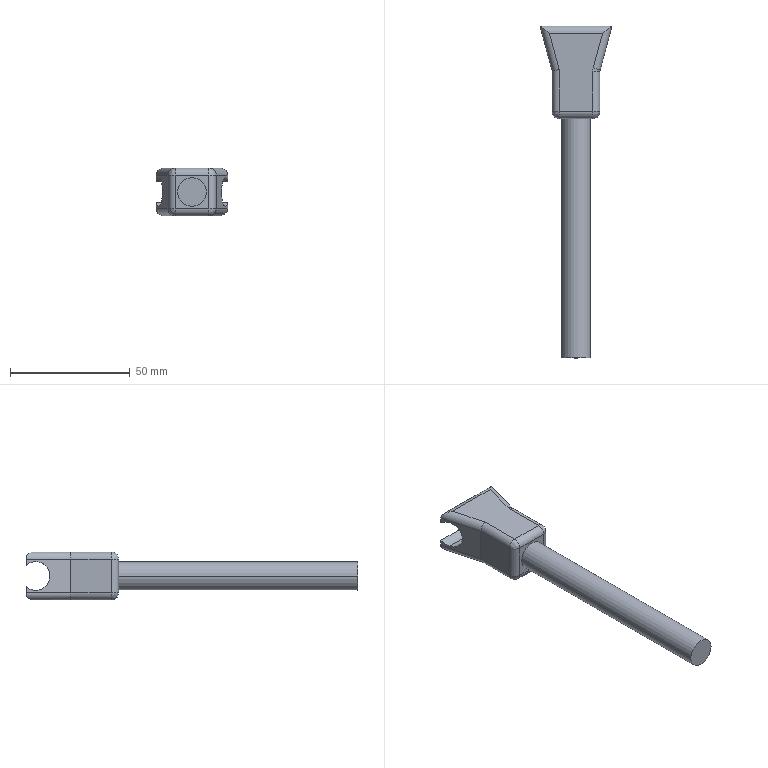Part | SolidWorks | features BaseBody 1 | 1 solid | 36 faces | box 30 x 138.66 x 20 mm | volume 25323 mm3 | cylinder 20 | plane 10 | spline 6 | commonest cylinder face diameters 6 x15 12 x5
STEP:
#1=CARTESIAN_POINT('',(-30.308,-117.701,10.));
#2=VERTEX_POINT('',#1);
#3=CARTESIAN_POINT('',(-18.308,-117.701,10.));
#4=VERTEX_POINT('',#3);
#5=CARTESIAN_POINT('',(-24.308,-117.701,10.));
#6=DIRECTION('',(0.,1.,0.));
#7=DIRECTION('',(-1.,0.,0.));
#8=AXIS2_PLACEMENT_3D('',#5,#6,#7);
#9=CIRCLE('',#8,6.);
#10=EDGE_CURVE('',#2,#4,#9,.T.);
#11=ORIENTED_EDGE('',*,*,#10,.T.);
#12=CARTESIAN_POINT('',(-18.308,-17.701,10.));
#13=VERTEX_POINT('',#12);
#14=CARTESIAN_POINT('',(-18.308,-117.701,10.));
#15=DIRECTION('',(0.,1.,0.));
#16=VECTOR('',#15,1000.);
#17=LINE('',#14,#16);
#18=EDGE_CURVE('',#4,#13,#17,.T.);
#19=ORIENTED_EDGE('',*,*,#18,.T.);
#20=CARTESIAN_POINT('',(-30.308,-17.701,10.));
#21=VERTEX_POINT('',#20);
#22=CARTESIAN_POINT('',(-24.308,-17.701,10.));
#23=DIRECTION('',(0.,-1.,0.));
#24=DIRECTION('',(-1.,0.,0.));
#25=AXIS2_PLACEMENT_3D('',#22,#23,#24);
#26=CIRCLE('',#25,6.);
#27=EDGE_CURVE('',#13,#21,#26,.T.);
#28=ORIENTED_EDGE('',*,*,#27,.T.);
#29=CARTESIAN_POINT('',(-30.308,-117.701,10.));
#30=DIRECTION('',(0.,1.,0.));
#31=VECTOR('',#30,1000.);
#32=LINE('',#29,#31);
#33=EDGE_CURVE('',#2,#21,#32,.T.);
#34=ORIENTED_EDGE('',*,*,#33,.F.);
#35=EDGE_LOOP('',(#11,#19,#28,#34));
#36=FACE_OUTER_BOUND('',#35,.T.);
#37=CARTESIAN_POINT('',(-24.308,-117.701,10.));
#38=DIRECTION('',(0.,1.,0.));
#39=DIRECTION('',(-1.,0.,0.));
#40=AXIS2_PLACEMENT_3D('',#37,#38,#39);
#41=CYLINDRICAL_SURFACE('',#40,6.);
#42=ADVANCED_FACE('',(#36),#41,.T.);
#43=CARTESIAN_POINT('',(-38.236,16.959,4.));
#44=VERTEX_POINT('',#43);
#45=CARTESIAN_POINT('',(-38.236,16.959,16.));
#46=VERTEX_POINT('',#45);
#47=CARTESIAN_POINT('',(-38.236,16.959,4.));
#48=CARTESIAN_POINT('',(-35.021,4.959,4.));
#49=CARTESIAN_POINT('',(-35.021,4.959,16.));
#50=CARTESIAN_POINT('',(-38.236,16.959,16.));
#51=(BOUNDED_CURVE()B_SPLINE_CURVE(3,(#47,#48,#49,#50),.UNSPECIFIED.,.F.,.F.)B_SPLINE_CURVE_WITH_KNOTS((4,4),(4.712,7.854),.UNSPECIFIED.)CURVE()GEOMETRIC_REPRESENTATION_ITEM()RATIONAL_B_SPLINE_CURVE((1.,0.3333,0.3333,1.))REPRESENTATION_ITEM(''));
#52=EDGE_CURVE('',#44,#46,#51,.T.);
#53=ORIENTED_EDGE('',*,*,#52,.T.);
#54=CARTESIAN_POINT('',(-10.38,16.959,16.));
#55=VERTEX_POINT('',#54);
#56=CARTESIAN_POINT('',(-100.,16.959,16.));
#57=DIRECTION('',(1.,0.,0.));
#58=VECTOR('',#57,1000.);
#59=LINE('',#56,#58);
#60=EDGE_CURVE('',#46,#55,#59,.T.);
#61=ORIENTED_EDGE('',*,*,#60,.T.);
#62=CARTESIAN_POINT('',(-10.38,16.959,4.));
#63=VERTEX_POINT('',#62);
#64=CARTESIAN_POINT('',(-10.38,16.959,16.));
#65=CARTESIAN_POINT('',(-13.595,4.959,16.));
#66=CARTESIAN_POINT('',(-13.595,4.959,4.));
#67=CARTESIAN_POINT('',(-10.38,16.959,4.));
#68=(BOUNDED_CURVE()B_SPLINE_CURVE(3,(#64,#65,#66,#67),.UNSPECIFIED.,.F.,.F.)B_SPLINE_CURVE_WITH_KNOTS((4,4),(1.571,4.712),.UNSPECIFIED.)CURVE()GEOMETRIC_REPRESENTATION_ITEM()RATIONAL_B_SPLINE_CURVE((1.,0.3333,0.3333,1.))REPRESENTATION_ITEM(''));
#69=EDGE_CURVE('',#55,#63,#68,.T.);
#70=ORIENTED_EDGE('',*,*,#69,.T.);
#71=CARTESIAN_POINT('',(-100.,16.959,4.));
#72=DIRECTION('',(1.,0.,0.));
#73=VECTOR('',#72,1000.);
#74=LINE('',#71,#73);
#75=EDGE_CURVE('',#44,#63,#74,.T.);
#76=ORIENTED_EDGE('',*,*,#75,.F.);
#77=EDGE_LOOP('',(#53,#61,#70,#76));
#78=FACE_OUTER_BOUND('',#77,.T.);
#79=CARTESIAN_POINT('',(-100.,16.959,10.));
#80=DIRECTION('',(1.,0.,0.));
#81=DIRECTION('',(0.,0.,-1.));
#82=AXIS2_PLACEMENT_3D('',#79,#80,#81);
#83=CYLINDRICAL_SURFACE('',#82,6.);
#84=ADVANCED_FACE('',(#78),#83,.F.);
#85=CARTESIAN_POINT('',(-39.308,20.959,5.528));
#86=VERTEX_POINT('',#85);
#87=CARTESIAN_POINT('',(-39.308,20.959,5.528));
#88=CARTESIAN_POINT('',(-39.01,19.847,4.533));
#89=CARTESIAN_POINT('',(-38.636,18.452,4.));
#90=CARTESIAN_POINT('',(-38.236,16.959,4.));
#91=(BOUNDED_CURVE()B_SPLINE_CURVE(3,(#87,#88,#89,#90),.UNSPECIFIED.,.F.,.T.)B_SPLINE_CURVE_WITH_KNOTS((4,4),(3.983,4.712),.UNSPECIFIED.)CURVE()GEOMETRIC_REPRESENTATION_ITEM()RATIONAL_B_SPLINE_CURVE((1.,0.9561,0.9561,1.))REPRESENTATION_ITEM(''));
#92=EDGE_CURVE('',#86,#44,#91,.T.);
#93=ORIENTED_EDGE('',*,*,#92,.T.);
#94=ORIENTED_EDGE('',*,*,#75,.T.);
#95=CARTESIAN_POINT('',(-9.308,20.959,5.528));
#96=VERTEX_POINT('',#95);
#97=CARTESIAN_POINT('',(-10.38,16.959,4.));
#98=CARTESIAN_POINT('',(-9.98,18.452,4.));
#99=CARTESIAN_POINT('',(-9.606,19.847,4.533));
#100=CARTESIAN_POINT('',(-9.308,20.959,5.528));
#101=(BOUNDED_CURVE()B_SPLINE_CURVE(3,(#97,#98,#99,#100),.UNSPECIFIED.,.F.,.F.)B_SPLINE_CURVE_WITH_KNOTS((4,4),(4.712,5.442),.UNSPECIFIED.)CURVE()GEOMETRIC_REPRESENTATION_ITEM()RATIONAL_B_SPLINE_CURVE((1.,0.9561,0.9561,1.))REPRESENTATION_ITEM(''));
#102=EDGE_CURVE('',#63,#96,#101,.T.);
#103=ORIENTED_EDGE('',*,*,#102,.T.);
#104=CARTESIAN_POINT('',(-39.308,20.959,5.528));
#105=DIRECTION('',(-1.,0.,0.));
#106=VECTOR('',#105,1000.);
#107=LINE('',#104,#106);
#108=EDGE_CURVE('',#96,#86,#107,.T.);
#109=ORIENTED_EDGE('',*,*,#108,.T.);
#110=EDGE_LOOP('',(#93,#94,#103,#109));
#111=FACE_OUTER_BOUND('',#110,.T.);
#112=CARTESIAN_POINT('',(-100.,16.959,10.));
#113=DIRECTION('',(1.,0.,0.));
#114=DIRECTION('',(0.,0.,-1.));
#115=AXIS2_PLACEMENT_3D('',#112,#113,#114);
#116=CYLINDRICAL_SURFACE('',#115,6.);
#117=ADVANCED_FACE('',(#111),#116,.F.);
#118=ORIENTED_EDGE('',*,*,#18,.F.);
#119=CARTESIAN_POINT('',(-24.308,-117.701,10.));
#120=DIRECTION('',(0.,1.,0.));
#121=DIRECTION('',(-1.,0.,0.));
#122=AXIS2_PLACEMENT_3D('',#119,#120,#121);
#123=CIRCLE('',#122,6.);
#124=EDGE_CURVE('',#4,#2,#123,.T.);
#125=ORIENTED_EDGE('',*,*,#124,.T.);
#126=ORIENTED_EDGE('',*,*,#33,.T.);
#127=CARTESIAN_POINT('',(-24.308,-17.701,10.));
#128=DIRECTION('',(0.,-1.,0.));
#129=DIRECTION('',(-1.,0.,0.));
#130=AXIS2_PLACEMENT_3D('',#127,#128,#129);
#131=CIRCLE('',#130,6.);
#132=EDGE_CURVE('',#21,#13,#131,.T.);
#133=ORIENTED_EDGE('',*,*,#132,.T.);
#134=EDGE_LOOP('',(#118,#125,#126,#133));
#135=FACE_OUTER_BOUND('',#134,.T.);
#136=CARTESIAN_POINT('',(-24.308,-117.701,10.));
#137=DIRECTION('',(0.,1.,0.));
#138=DIRECTION('',(-1.,0.,0.));
#139=AXIS2_PLACEMENT_3D('',#136,#137,#138);
#140=CYLINDRICAL_SURFACE('',#139,6.);
#141=ADVANCED_FACE('',(#135),#140,.T.);
#142=ORIENTED_EDGE('',*,*,#132,.F.);
#143=ORIENTED_EDGE('',*,*,#27,.F.);
#144=EDGE_LOOP('',(#142,#143));
#145=FACE_BOUND('',#144,.T.);
#146=CARTESIAN_POINT('',(-31.308,-17.701,3.));
#147=VERTEX_POINT('',#146);
#148=CARTESIAN_POINT('',(-31.308,-17.701,17.));
#149=VERTEX_POINT('',#148);
#150=CARTESIAN_POINT('',(-31.308,-17.701,20.));
#151=DIRECTION('',(0.,0.,1.));
#152=VECTOR('',#151,1000.);
#153=LINE('',#150,#152);
#154=EDGE_CURVE('',#147,#149,#153,.T.);
#155=ORIENTED_EDGE('',*,*,#154,.F.);
#156=CARTESIAN_POINT('',(-17.308,-17.701,3.));
#157=VERTEX_POINT('',#156);
#158=CARTESIAN_POINT('',(-14.308,-17.701,3.));
#159=DIRECTION('',(-1.,0.,0.));
#160=VECTOR('',#159,1000.);
#161=LINE('',#158,#160);
#162=EDGE_CURVE('',#157,#147,#161,.T.);
#163=ORIENTED_EDGE('',*,*,#162,.F.);
#164=CARTESIAN_POINT('',(-17.308,-17.701,17.));
#165=VERTEX_POINT('',#164);
#166=CARTESIAN_POINT('',(-17.308,-17.701,20.));
#167=DIRECTION('',(0.,0.,-1.));
#168=VECTOR('',#167,1000.);
#169=LINE('',#166,#168);
#170=EDGE_CURVE('',#165,#157,#169,.T.);
#171=ORIENTED_EDGE('',*,*,#170,.F.);
#172=CARTESIAN_POINT('',(-14.308,-17.701,17.));
#173=DIRECTION('',(1.,0.,0.));
#174=VECTOR('',#173,1000.);
#175=LINE('',#172,#174);
#176=EDGE_CURVE('',#149,#165,#175,.T.);
#177=ORIENTED_EDGE('',*,*,#176,.F.);
#178=EDGE_LOOP('',(#155,#163,#171,#177));
#179=FACE_OUTER_BOUND('',#178,.T.);
#180=CARTESIAN_POINT('',(-14.308,-17.701,20.));
#181=DIRECTION('',(0.,1.,0.));
#182=DIRECTION('',(-1.,0.,0.));
#183=AXIS2_PLACEMENT_3D('',#180,#181,#182);
#184=PLANE('',#183);
#185=ADVANCED_FACE('',(#145,#179),#184,.F.);
#186=ORIENTED_EDGE('',*,*,#10,.F.);
#187=ORIENTED_EDGE('',*,*,#124,.F.);
#188=EDGE_LOOP('',(#186,#187));
#189=FACE_OUTER_BOUND('',#188,.T.);
#190=CARTESIAN_POINT('',(-24.308,-117.701,10.));
#191=DIRECTION('',(0.,-1.,0.));
#192=DIRECTION('',(1.,0.,0.));
#193=AXIS2_PLACEMENT_3D('',#190,#191,#192);
#194=PLANE('',#193);
#195=ADVANCED_FACE('',(#189),#194,.T.);
#196=CARTESIAN_POINT('',(-17.308,-14.701,20.));
#197=VERTEX_POINT('',#196);
#198=CARTESIAN_POINT('',(-17.308,-14.701,17.));
#199=DIRECTION('',(-1.,0.,0.));
#200=DIRECTION('',(0.,1.,0.));
#201=AXIS2_PLACEMENT_3D('',#198,#199,#200);
#202=CIRCLE('',#201,3.);
#203=EDGE_CURVE('',#165,#197,#202,.T.);
#204=ORIENTED_EDGE('',*,*,#203,.T.);
#205=CARTESIAN_POINT('',(-31.308,-14.701,20.));
#206=VERTEX_POINT('',#205);
#207=CARTESIAN_POINT('',(0.,-14.701,20.));
#208=DIRECTION('',(-1.,0.,0.));
#209=VECTOR('',#208,1000.);
#210=LINE('',#207,#209);
#211=EDGE_CURVE('',#197,#206,#210,.T.);
#212=ORIENTED_EDGE('',*,*,#211,.T.);
#213=CARTESIAN_POINT('',(-31.308,-14.701,17.));
#214=DIRECTION('',(1.,0.,0.));
#215=DIRECTION('',(0.,1.,0.));
#216=AXIS2_PLACEMENT_3D('',#213,#214,#215);
#217=CIRCLE('',#216,3.);
#218=EDGE_CURVE('',#206,#149,#217,.T.);
#219=ORIENTED_EDGE('',*,*,#218,.T.);
#220=ORIENTED_EDGE('',*,*,#176,.T.);
#221=EDGE_LOOP('',(#204,#212,#219,#220));
#222=FACE_OUTER_BOUND('',#221,.T.);
#223=CARTESIAN_POINT('',(0.,-14.701,17.));
#224=DIRECTION('',(1.,0.,0.));
#225=DIRECTION('',(0.,1.,0.));
#226=AXIS2_PLACEMENT_3D('',#223,#224,#225);
#227=CYLINDRICAL_SURFACE('',#226,3.);
#228=ADVANCED_FACE('',(#222),#227,.T.);
#229=CARTESIAN_POINT('',(-34.308,-14.701,17.));
#230=VERTEX_POINT('',#229);
#231=CARTESIAN_POINT('',(-31.308,-14.701,17.));
#232=DIRECTION('',(0.,0.,-1.));
#233=DIRECTION('',(-1.,0.,0.));
#234=AXIS2_PLACEMENT_3D('',#231,#232,#233);
#235=CIRCLE('',#234,3.);
#236=EDGE_CURVE('',#149,#230,#235,.T.);
#237=ORIENTED_EDGE('',*,*,#236,.T.);
#238=CARTESIAN_POINT('',(-34.308,-14.701,3.));
#239=VERTEX_POINT('',#238);
#240=CARTESIAN_POINT('',(-34.308,-14.701,20.));
#241=DIRECTION('',(0.,0.,-1.));
#242=VECTOR('',#241,1000.);
#243=LINE('',#240,#242);
#244=EDGE_CURVE('',#230,#239,#243,.T.);
#245=ORIENTED_EDGE('',*,*,#244,.T.);
#246=CARTESIAN_POINT('',(-31.308,-14.701,3.));
#247=DIRECTION('',(0.,0.,1.));
#248=DIRECTION('',(-1.,0.,0.));
#249=AXIS2_PLACEMENT_3D('',#246,#247,#248);
#250=CIRCLE('',#249,3.);
#251=EDGE_CURVE('',#239,#147,#250,.T.);
#252=ORIENTED_EDGE('',*,*,#251,.T.);
#253=ORIENTED_EDGE('',*,*,#154,.T.);
#254=EDGE_LOOP('',(#237,#245,#252,#253));
#255=FACE_OUTER_BOUND('',#254,.T.);
#256=CARTESIAN_POINT('',(-31.308,-14.701,20.));
#257=DIRECTION('',(0.,0.,-1.));
#258=DIRECTION('',(-1.,0.,0.));
#259=AXIS2_PLACEMENT_3D('',#256,#257,#258);
#260=CYLINDRICAL_SURFACE('',#259,3.);
#261=ADVANCED_FACE('',(#255),#260,.T.);
#262=CARTESIAN_POINT('',(-17.308,-14.701,0.));
#263=VERTEX_POINT('',#262);
#264=CARTESIAN_POINT('',(-17.308,-14.701,3.));
#265=DIRECTION('',(-1.,0.,0.));
#266=DIRECTION('',(0.,-1.,0.));
#267=AXIS2_PLACEMENT_3D('',#264,#265,#266);
#268=CIRCLE('',#267,3.);
#269=EDGE_CURVE('',#263,#157,#268,.T.);
#270=ORIENTED_EDGE('',*,*,#269,.T.);
#271=ORIENTED_EDGE('',*,*,#162,.T.);
#272=CARTESIAN_POINT('',(-31.308,-14.701,0.));
#273=VERTEX_POINT('',#272);
#274=CARTESIAN_POINT('',(-31.308,-14.701,3.));
#275=DIRECTION('',(1.,0.,0.));
#276=DIRECTION('',(0.,-1.,0.));
#277=AXIS2_PLACEMENT_3D('',#274,#275,#276);
#278=CIRCLE('',#277,3.);
#279=EDGE_CURVE('',#147,#273,#278,.T.);
#280=ORIENTED_EDGE('',*,*,#279,.T.);
#281=CARTESIAN_POINT('',(-14.308,-14.701,0.));
#282=DIRECTION('',(1.,0.,0.));
#283=VECTOR('',#282,1000.);
#284=LINE('',#281,#283);
#285=EDGE_CURVE('',#273,#263,#284,.T.);
#286=ORIENTED_EDGE('',*,*,#285,.T.);
#287=EDGE_LOOP('',(#270,#271,#280,#286));
#288=FACE_OUTER_BOUND('',#287,.T.);
#289=CARTESIAN_POINT('',(-14.308,-14.701,3.));
#290=DIRECTION('',(-1.,0.,0.));
#291=DIRECTION('',(0.,-1.,0.));
#292=AXIS2_PLACEMENT_3D('',#289,#290,#291);
#293=CYLINDRICAL_SURFACE('',#292,3.);
#294=ADVANCED_FACE('',(#288),#293,.T.);
#295=CARTESIAN_POINT('',(-14.308,-14.701,17.));
#296=VERTEX_POINT('',#295);
#297=CARTESIAN_POINT('',(-17.308,-14.701,17.));
#298=DIRECTION('',(0.,0.,-1.));
#299=DIRECTION('',(-1.,0.,0.));
#300=AXIS2_PLACEMENT_3D('',#297,#298,#299);
#301=CIRCLE('',#300,3.);
#302=EDGE_CURVE('',#296,#165,#301,.T.);
#303=ORIENTED_EDGE('',*,*,#302,.T.);
#304=ORIENTED_EDGE('',*,*,#170,.T.);
#305=CARTESIAN_POINT('',(-14.308,-14.701,3.));
#306=VERTEX_POINT('',#305);
#307=CARTESIAN_POINT('',(-17.308,-14.701,3.));
#308=DIRECTION('',(0.,0.,1.));
#309=DIRECTION('',(-1.,0.,0.));
#310=AXIS2_PLACEMENT_3D('',#307,#308,#309);
#311=CIRCLE('',#310,3.);
#312=EDGE_CURVE('',#157,#306,#311,.T.);
#313=ORIENTED_EDGE('',*,*,#312,.T.);
#314=CARTESIAN_POINT('',(-14.308,-14.701,20.));
#315=DIRECTION('',(0.,0.,1.));
#316=VECTOR('',#315,1000.);
#317=LINE('',#314,#316);
#318=EDGE_CURVE('',#306,#296,#317,.T.);
#319=ORIENTED_EDGE('',*,*,#318,.T.);
#320=EDGE_LOOP('',(#303,#304,#313,#319));
#321=FACE_OUTER_BOUND('',#320,.T.);
#322=CARTESIAN_POINT('',(-17.308,-14.701,20.));
#323=DIRECTION('',(0.,0.,-1.));
#324=DIRECTION('',(-1.,0.,0.));
#325=AXIS2_PLACEMENT_3D('',#322,#323,#324);
#326=CYLINDRICAL_SURFACE('',#325,3.);
#327=ADVANCED_FACE('',(#321),#326,.T.);
#328=CARTESIAN_POINT('',(-13.218,17.959,20.));
#329=VERTEX_POINT('',#328);
#330=CARTESIAN_POINT('',(-17.104,3.457,20.));
#331=VERTEX_POINT('',#330);
#332=CARTESIAN_POINT('',(-13.218,17.959,20.));
#333=DIRECTION('',(-0.2588,-0.9659,0.));
#334=VECTOR('',#333,1000.);
#335=LINE('',#332,#334);
#336=EDGE_CURVE('',#329,#331,#335,.T.);
#337=ORIENTED_EDGE('',*,*,#336,.F.);
#338=CARTESIAN_POINT('',(-35.399,17.959,20.));
#339=VERTEX_POINT('',#338);
#340=CARTESIAN_POINT('',(0.,17.959,20.));
#341=DIRECTION('',(1.,0.,0.));
#342=VECTOR('',#341,1000.);
#343=LINE('',#340,#342);
#344=EDGE_CURVE('',#339,#329,#343,.T.);
#345=ORIENTED_EDGE('',*,*,#344,.F.);
#346=CARTESIAN_POINT('',(-31.308,2.694,20.));
#347=VERTEX_POINT('',#346);
#348=CARTESIAN_POINT('',(-31.308,2.694,20.));
#349=DIRECTION('',(-0.2588,0.9659,0.));
#350=VECTOR('',#349,1000.);
#351=LINE('',#348,#350);
#352=EDGE_CURVE('',#347,#339,#351,.T.);
#353=ORIENTED_EDGE('',*,*,#352,.F.);
#354=CARTESIAN_POINT('',(-31.308,0.,20.));
#355=DIRECTION('',(0.,1.,0.));
#356=VECTOR('',#355,1000.);
#357=LINE('',#354,#356);
#358=EDGE_CURVE('',#206,#347,#357,.T.);
#359=ORIENTED_EDGE('',*,*,#358,.F.);
#360=ORIENTED_EDGE('',*,*,#211,.F.);
#361=CARTESIAN_POINT('',(-17.308,1.904,20.));
#362=VERTEX_POINT('',#361);
#363=CARTESIAN_POINT('',(-17.308,0.,20.));
#364=DIRECTION('',(0.,-1.,0.));
#365=VECTOR('',#364,1000.);
#366=LINE('',#363,#365);
#367=EDGE_CURVE('',#362,#197,#366,.T.);
#368=ORIENTED_EDGE('',*,*,#367,.F.);
#369=CARTESIAN_POINT('',(-17.104,3.457,20.));
#370=CARTESIAN_POINT('',(-17.24,2.95,20.));
#371=CARTESIAN_POINT('',(-17.308,2.429,20.));
#372=CARTESIAN_POINT('',(-17.308,1.904,20.));
#373=(BOUNDED_CURVE()B_SPLINE_CURVE(3,(#369,#370,#371,#372),.UNSPECIFIED.,.F.,.F.)B_SPLINE_CURVE_WITH_KNOTS((4,4),(0.,1.),.UNSPECIFIED.)CURVE()GEOMETRIC_REPRESENTATION_ITEM()RATIONAL_B_SPLINE_CURVE((1.,0.9943,0.9943,1.))REPRESENTATION_ITEM(''));
#374=EDGE_CURVE('',#331,#362,#373,.T.);
#375=ORIENTED_EDGE('',*,*,#374,.F.);
#376=EDGE_LOOP('',(#337,#345,#353,#359,#360,#368,#375));
#377=FACE_OUTER_BOUND('',#376,.T.);
#378=CARTESIAN_POINT('',(0.,0.,20.));
#379=DIRECTION('',(0.,0.,-1.));
#380=DIRECTION('',(-1.,0.,0.));
#381=AXIS2_PLACEMENT_3D('',#378,#379,#380);
#382=PLANE('',#381);
#383=ADVANCED_FACE('',(#377),#382,.F.);
#384=ORIENTED_EDGE('',*,*,#302,.F.);
#385=CARTESIAN_POINT('',(-17.308,-14.701,17.));
#386=DIRECTION('',(0.,-1.,0.));
#387=DIRECTION('',(1.,0.,0.));
#388=AXIS2_PLACEMENT_3D('',#385,#386,#387);
#389=CIRCLE('',#388,3.);
#390=EDGE_CURVE('',#296,#197,#389,.T.);
#391=ORIENTED_EDGE('',*,*,#390,.T.);
#392=ORIENTED_EDGE('',*,*,#203,.F.);
#393=EDGE_LOOP('',(#384,#391,#392));
#394=FACE_OUTER_BOUND('',#393,.T.);
#395=CARTESIAN_POINT('',(-14.308,-14.701,17.));
#396=CARTESIAN_POINT('',(-14.308,-14.701,17.));
#397=CARTESIAN_POINT('',(-14.308,-14.701,17.));
#398=CARTESIAN_POINT('',(-14.308,-14.701,17.));
#399=CARTESIAN_POINT('',(-14.308,-14.701,18.757));
#400=CARTESIAN_POINT('',(-14.308,-15.73,18.757));
#401=CARTESIAN_POINT('',(-14.308,-16.458,18.029));
#402=CARTESIAN_POINT('',(-14.308,-16.458,17.));
#403=CARTESIAN_POINT('',(-15.551,-14.701,20.));
#404=CARTESIAN_POINT('',(-15.551,-16.458,20.));
#405=CARTESIAN_POINT('',(-15.551,-17.701,18.757));
#406=CARTESIAN_POINT('',(-15.551,-17.701,17.));
#407=CARTESIAN_POINT('',(-17.308,-14.701,20.));
#408=CARTESIAN_POINT('',(-17.308,-16.458,20.));
#409=CARTESIAN_POINT('',(-17.308,-17.701,18.757));
#410=CARTESIAN_POINT('',(-17.308,-17.701,17.));
#411=(BOUNDED_SURFACE()B_SPLINE_SURFACE(3,3,((#395,#396,#397,#398),(#399,#400,#401,#402),(#403,#404,#405,#406),(#407,#408,#409,#410)),.UNSPECIFIED.,.F.,.F.,.T.)B_SPLINE_SURFACE_WITH_KNOTS((4,4),(4,4),(0.,1.),(0.,1.),.UNSPECIFIED.)GEOMETRIC_REPRESENTATION_ITEM()RATIONAL_B_SPLINE_SURFACE(((1.,0.8047,0.8047,1.),(0.8047,0.6476,0.6476,0.8047),(0.8047,0.6476,0.6476,0.8047),(1.,0.8047,0.8047,1.)))REPRESENTATION_ITEM('')SURFACE());
#412=ADVANCED_FACE('',(#394),#411,.T.);
#413=ORIENTED_EDGE('',*,*,#218,.F.);
#414=CARTESIAN_POINT('',(-31.308,-14.701,17.));
#415=DIRECTION('',(0.,-1.,0.));
#416=DIRECTION('',(1.,0.,0.));
#417=AXIS2_PLACEMENT_3D('',#414,#415,#416);
#418=CIRCLE('',#417,3.);
#419=EDGE_CURVE('',#206,#230,#418,.T.);
#420=ORIENTED_EDGE('',*,*,#419,.T.);
#421=ORIENTED_EDGE('',*,*,#236,.F.);
#422=EDGE_LOOP('',(#413,#420,#421));
#423=FACE_OUTER_BOUND('',#422,.T.);
#424=CARTESIAN_POINT('',(-31.308,-14.701,20.));
#425=CARTESIAN_POINT('',(-31.308,-16.458,20.));
#426=CARTESIAN_POINT('',(-31.308,-17.701,18.757));
#427=CARTESIAN_POINT('',(-31.308,-17.701,17.));
#428=CARTESIAN_POINT('',(-33.066,-14.701,20.));
#429=CARTESIAN_POINT('',(-33.066,-16.458,20.));
#430=CARTESIAN_POINT('',(-33.066,-17.701,18.757));
#431=CARTESIAN_POINT('',(-33.066,-17.701,17.));
#432=CARTESIAN_POINT('',(-34.308,-14.701,18.757));
#433=CARTESIAN_POINT('',(-34.308,-15.73,18.757));
#434=CARTESIAN_POINT('',(-34.308,-16.458,18.029));
#435=CARTESIAN_POINT('',(-34.308,-16.458,17.));
#436=CARTESIAN_POINT('',(-34.308,-14.701,17.));
#437=CARTESIAN_POINT('',(-34.308,-14.701,17.));
#438=CARTESIAN_POINT('',(-34.308,-14.701,17.));
#439=CARTESIAN_POINT('',(-34.308,-14.701,17.));
#440=(BOUNDED_SURFACE()B_SPLINE_SURFACE(3,3,((#424,#425,#426,#427),(#428,#429,#430,#431),(#432,#433,#434,#435),(#436,#437,#438,#439)),.UNSPECIFIED.,.F.,.F.,.F.)B_SPLINE_SURFACE_WITH_KNOTS((4,4),(4,4),(0.,1.),(0.,1.),.UNSPECIFIED.)GEOMETRIC_REPRESENTATION_ITEM()RATIONAL_B_SPLINE_SURFACE(((1.,0.8047,0.8047,1.),(0.8047,0.6476,0.6476,0.8047),(0.8047,0.6476,0.6476,0.8047),(1.,0.8047,0.8047,1.)))REPRESENTATION_ITEM('')SURFACE());
#441=ADVANCED_FACE('',(#423),#440,.T.);
#442=CARTESIAN_POINT('',(-34.308,2.299,17.));
#443=VERTEX_POINT('',#442);
#444=CARTESIAN_POINT('',(-34.308,-17.701,17.));
#445=DIRECTION('',(0.,-1.,0.));
#446=VECTOR('',#445,1000.);
#447=LINE('',#444,#446);
#448=EDGE_CURVE('',#443,#230,#447,.T.);
#449=ORIENTED_EDGE('',*,*,#448,.F.);
#450=CARTESIAN_POINT('',(-34.308,2.299,3.));
#451=VERTEX_POINT('',#450);
#452=CARTESIAN_POINT('',(-34.308,2.299,20.));
#453=DIRECTION('',(0.,0.,1.));
#454=VECTOR('',#453,1000.);
#455=LINE('',#452,#454);
#456=EDGE_CURVE('',#451,#443,#455,.T.);
#457=ORIENTED_EDGE('',*,*,#456,.F.);
#458=CARTESIAN_POINT('',(-34.308,-17.701,3.));
#459=DIRECTION('',(0.,1.,0.));
#460=VECTOR('',#459,1000.);
#461=LINE('',#458,#460);
#462=EDGE_CURVE('',#239,#451,#461,.T.);
#463=ORIENTED_EDGE('',*,*,#462,.F.);
#464=ORIENTED_EDGE('',*,*,#244,.F.);
#465=EDGE_LOOP('',(#449,#457,#463,#464));
#466=FACE_OUTER_BOUND('',#465,.T.);
#467=CARTESIAN_POINT('',(-34.308,-17.701,20.));
#468=DIRECTION('',(1.,0.,0.));
#469=DIRECTION('',(0.,0.,-1.));
#470=AXIS2_PLACEMENT_3D('',#467,#468,#469);
#471=PLANE('',#470);
#472=ADVANCED_FACE('',(#466),#471,.F.);
#473=ORIENTED_EDGE('',*,*,#279,.F.);
#474=ORIENTED_EDGE('',*,*,#251,.F.);
#475=CARTESIAN_POINT('',(-31.308,-14.701,3.));
#476=DIRECTION('',(0.,-1.,0.));
#477=DIRECTION('',(1.,0.,0.));
#478=AXIS2_PLACEMENT_3D('',#475,#476,#477);
#479=CIRCLE('',#478,3.);
#480=EDGE_CURVE('',#239,#273,#479,.T.);
#481=ORIENTED_EDGE('',*,*,#480,.T.);
#482=EDGE_LOOP('',(#473,#474,#481));
#483=FACE_OUTER_BOUND('',#482,.T.);
#484=CARTESIAN_POINT('',(-31.308,-17.701,3.));
#485=CARTESIAN_POINT('',(-31.308,-17.701,1.243));
#486=CARTESIAN_POINT('',(-31.308,-16.458,0.));
#487=CARTESIAN_POINT('',(-31.308,-14.701,0.));
#488=CARTESIAN_POINT('',(-33.066,-17.701,3.));
#489=CARTESIAN_POINT('',(-33.066,-17.701,1.243));
#490=CARTESIAN_POINT('',(-33.066,-16.458,0.));
#491=CARTESIAN_POINT('',(-33.066,-14.701,0.));
#492=CARTESIAN_POINT('',(-34.308,-16.458,3.));
#493=CARTESIAN_POINT('',(-34.308,-16.458,1.971));
#494=CARTESIAN_POINT('',(-34.308,-15.73,1.243));
#495=CARTESIAN_POINT('',(-34.308,-14.701,1.243));
#496=CARTESIAN_POINT('',(-34.308,-14.701,3.));
#497=CARTESIAN_POINT('',(-34.308,-14.701,3.));
#498=CARTESIAN_POINT('',(-34.308,-14.701,3.));
#499=CARTESIAN_POINT('',(-34.308,-14.701,3.));
#500=(BOUNDED_SURFACE()B_SPLINE_SURFACE(3,3,((#484,#485,#486,#487),(#488,#489,#490,#491),(#492,#493,#494,#495),(#496,#497,#498,#499)),.UNSPECIFIED.,.F.,.F.,.T.)B_SPLINE_SURFACE_WITH_KNOTS((4,4),(4,4),(0.,1.),(0.,1.),.UNSPECIFIED.)GEOMETRIC_REPRESENTATION_ITEM()RATIONAL_B_SPLINE_SURFACE(((1.,0.8047,0.8047,1.),(0.8047,0.6476,0.6476,0.8047),(0.8047,0.6476,0.6476,0.8047),(1.,0.8047,0.8047,1.)))REPRESENTATION_ITEM('')SURFACE());
#501=ADVANCED_FACE('',(#483),#500,.T.);
#502=ORIENTED_EDGE('',*,*,#269,.F.);
#503=CARTESIAN_POINT('',(-17.308,-14.701,3.));
#504=DIRECTION('',(0.,-1.,0.));
#505=DIRECTION('',(1.,0.,0.));
#506=AXIS2_PLACEMENT_3D('',#503,#504,#505);
#507=CIRCLE('',#506,3.);
#508=EDGE_CURVE('',#263,#306,#507,.T.);
#509=ORIENTED_EDGE('',*,*,#508,.T.);
#510=ORIENTED_EDGE('',*,*,#312,.F.);
#511=EDGE_LOOP('',(#502,#509,#510));
#512=FACE_OUTER_BOUND('',#511,.T.);
#513=CARTESIAN_POINT('',(-14.308,-14.701,3.));
#514=CARTESIAN_POINT('',(-14.308,-14.701,3.));
#515=CARTESIAN_POINT('',(-14.308,-14.701,3.));
#516=CARTESIAN_POINT('',(-14.308,-14.701,3.));
#517=CARTESIAN_POINT('',(-14.308,-16.458,3.));
#518=CARTESIAN_POINT('',(-14.308,-16.458,1.971));
#519=CARTESIAN_POINT('',(-14.308,-15.73,1.243));
#520=CARTESIAN_POINT('',(-14.308,-14.701,1.243));
#521=CARTESIAN_POINT('',(-15.551,-17.701,3.));
#522=CARTESIAN_POINT('',(-15.551,-17.701,1.243));
#523=CARTESIAN_POINT('',(-15.551,-16.458,0.));
#524=CARTESIAN_POINT('',(-15.551,-14.701,0.));
#525=CARTESIAN_POINT('',(-17.308,-17.701,3.));
#526=CARTESIAN_POINT('',(-17.308,-17.701,1.243));
#527=CARTESIAN_POINT('',(-17.308,-16.458,0.));
#528=CARTESIAN_POINT('',(-17.308,-14.701,0.));
#529=(BOUNDED_SURFACE()B_SPLINE_SURFACE(3,3,((#513,#514,#515,#516),(#517,#518,#519,#520),(#521,#522,#523,#524),(#525,#526,#527,#528)),.UNSPECIFIED.,.F.,.F.,.F.)B_SPLINE_SURFACE_WITH_KNOTS((4,4),(4,4),(0.,1.),(0.,1.),.UNSPECIFIED.)GEOMETRIC_REPRESENTATION_ITEM()RATIONAL_B_SPLINE_SURFACE(((1.,0.8047,0.8047,1.),(0.8047,0.6476,0.6476,0.8047),(0.8047,0.6476,0.6476,0.8047),(1.,0.8047,0.8047,1.)))REPRESENTATION_ITEM('')SURFACE());
#530=ADVANCED_FACE('',(#512),#529,.T.);
#531=CARTESIAN_POINT('',(-31.308,2.694,0.));
#532=VERTEX_POINT('',#531);
#533=CARTESIAN_POINT('',(-31.308,0.,0.));
#534=DIRECTION('',(0.,1.,0.));
#535=VECTOR('',#534,1000.);
#536=LINE('',#533,#535);
#537=EDGE_CURVE('',#273,#532,#536,.T.);
#538=ORIENTED_EDGE('',*,*,#537,.T.);
#539=CARTESIAN_POINT('',(-35.399,17.959,0.));
#540=VERTEX_POINT('',#539);
#541=CARTESIAN_POINT('',(-31.308,2.694,0.));
#542=DIRECTION('',(-0.2588,0.9659,0.));
#543=VECTOR('',#542,1000.);
#544=LINE('',#541,#543);
#545=EDGE_CURVE('',#532,#540,#544,.T.);
#546=ORIENTED_EDGE('',*,*,#545,.T.);
#547=CARTESIAN_POINT('',(-13.218,17.959,0.));
#548=VERTEX_POINT('',#547);
#549=CARTESIAN_POINT('',(0.,17.959,0.));
#550=DIRECTION('',(1.,0.,0.));
#551=VECTOR('',#550,1000.);
#552=LINE('',#549,#551);
#553=EDGE_CURVE('',#540,#548,#552,.T.);
#554=ORIENTED_EDGE('',*,*,#553,.T.);
#555=CARTESIAN_POINT('',(-17.104,3.457,0.));
#556=VERTEX_POINT('',#555);
#557=CARTESIAN_POINT('',(-13.218,17.959,0.));
#558=DIRECTION('',(-0.2588,-0.9659,0.));
#559=VECTOR('',#558,1000.);
#560=LINE('',#557,#559);
#561=EDGE_CURVE('',#548,#556,#560,.T.);
#562=ORIENTED_EDGE('',*,*,#561,.T.);
#563=CARTESIAN_POINT('',(-17.308,1.904,0.));
#564=VERTEX_POINT('',#563);
#565=CARTESIAN_POINT('',(-17.308,1.904,0.));
#566=CARTESIAN_POINT('',(-17.308,2.429,0.));
#567=CARTESIAN_POINT('',(-17.24,2.95,0.));
#568=CARTESIAN_POINT('',(-17.104,3.457,0.));
#569=(BOUNDED_CURVE()B_SPLINE_CURVE(3,(#565,#566,#567,#568),.UNSPECIFIED.,.F.,.F.)B_SPLINE_CURVE_WITH_KNOTS((4,4),(0.,1.),.UNSPECIFIED.)CURVE()GEOMETRIC_REPRESENTATION_ITEM()RATIONAL_B_SPLINE_CURVE((1.,0.9943,0.9943,1.))REPRESENTATION_ITEM(''));
#570=EDGE_CURVE('',#564,#556,#569,.T.);
#571=ORIENTED_EDGE('',*,*,#570,.F.);
#572=CARTESIAN_POINT('',(-17.308,0.,0.));
#573=DIRECTION('',(0.,-1.,0.));
#574=VECTOR('',#573,1000.);
#575=LINE('',#572,#574);
#576=EDGE_CURVE('',#564,#263,#575,.T.);
#577=ORIENTED_EDGE('',*,*,#576,.T.);
#578=ORIENTED_EDGE('',*,*,#285,.F.);
#579=EDGE_LOOP('',(#538,#546,#554,#562,#571,#577,#578));
#580=FACE_OUTER_BOUND('',#579,.T.);
#581=CARTESIAN_POINT('',(0.,0.,0.));
#582=DIRECTION('',(0.,0.,-1.));
#583=DIRECTION('',(-1.,0.,0.));
#584=AXIS2_PLACEMENT_3D('',#581,#582,#583);
#585=PLANE('',#584);
#586=ADVANCED_FACE('',(#580),#585,.T.);
#587=ORIENTED_EDGE('',*,*,#318,.F.);
#588=CARTESIAN_POINT('',(-14.308,1.904,3.));
#589=VERTEX_POINT('',#588);
#590=CARTESIAN_POINT('',(-14.308,2.299,3.));
#591=DIRECTION('',(0.,-1.,0.));
#592=VECTOR('',#591,1000.);
#593=LINE('',#590,#592);
#594=EDGE_CURVE('',#589,#306,#593,.T.);
#595=ORIENTED_EDGE('',*,*,#594,.F.);
#596=CARTESIAN_POINT('',(-14.308,1.904,17.));
#597=VERTEX_POINT('',#596);
#598=CARTESIAN_POINT('',(-14.308,1.904,20.));
#599=DIRECTION('',(0.,0.,-1.));
#600=VECTOR('',#599,1000.);
#601=LINE('',#598,#600);
#602=EDGE_CURVE('',#597,#589,#601,.T.);
#603=ORIENTED_EDGE('',*,*,#602,.F.);
#604=CARTESIAN_POINT('',(-14.308,2.299,17.));
#605=DIRECTION('',(0.,1.,0.));
#606=VECTOR('',#605,1000.);
#607=LINE('',#604,#606);
#608=EDGE_CURVE('',#296,#597,#607,.T.);
#609=ORIENTED_EDGE('',*,*,#608,.F.);
#610=EDGE_LOOP('',(#587,#595,#603,#609));
#611=FACE_OUTER_BOUND('',#610,.T.);
#612=CARTESIAN_POINT('',(-14.308,2.299,20.));
#613=DIRECTION('',(-1.,0.,0.));
#614=DIRECTION('',(0.,-1.,0.));
#615=AXIS2_PLACEMENT_3D('',#612,#613,#614);
#616=PLANE('',#615);
#617=ADVANCED_FACE('',(#611),#616,.F.);
#618=CARTESIAN_POINT('',(-9.308,20.959,17.));
#619=VERTEX_POINT('',#618);
#620=CARTESIAN_POINT('',(-9.308,20.959,17.));
#621=CARTESIAN_POINT('',(-9.308,20.959,18.757));
#622=CARTESIAN_POINT('',(-10.928,19.717,20.));
#623=CARTESIAN_POINT('',(-13.218,17.959,20.));
#624=(BOUNDED_CURVE()B_SPLINE_CURVE(3,(#620,#621,#622,#623),.UNSPECIFIED.,.F.,.F.)B_SPLINE_CURVE_WITH_KNOTS((4,4),(0.,1.571),.UNSPECIFIED.)CURVE()GEOMETRIC_REPRESENTATION_ITEM()RATIONAL_B_SPLINE_CURVE((1.,0.8047,0.8047,1.))REPRESENTATION_ITEM(''));
#625=EDGE_CURVE('',#619,#329,#624,.T.);
#626=ORIENTED_EDGE('',*,*,#625,.T.);
#627=ORIENTED_EDGE('',*,*,#336,.T.);
#628=CARTESIAN_POINT('',(-14.206,2.68,17.));
#629=VERTEX_POINT('',#628);
#630=CARTESIAN_POINT('',(-17.104,3.457,17.));
#631=DIRECTION('',(0.2588,0.9659,0.));
#632=DIRECTION('',(-0.9659,0.2588,0.));
#633=AXIS2_PLACEMENT_3D('',#630,#631,#632);
#634=CIRCLE('',#633,3.);
#635=EDGE_CURVE('',#331,#629,#634,.T.);
#636=ORIENTED_EDGE('',*,*,#635,.T.);
#637=CARTESIAN_POINT('',(-13.924,3.731,17.));
#638=DIRECTION('',(0.2588,0.9659,0.));
#639=VECTOR('',#638,1000.);
#640=LINE('',#637,#639);
#641=EDGE_CURVE('',#629,#619,#640,.T.);
#642=ORIENTED_EDGE('',*,*,#641,.T.);
#643=EDGE_LOOP('',(#626,#627,#636,#642));
#644=FACE_OUTER_BOUND('',#643,.T.);
#645=CARTESIAN_POINT('',(-16.822,4.508,17.));
#646=DIRECTION('',(0.2588,0.9659,0.));
#647=DIRECTION('',(-0.9659,0.2588,0.));
#648=AXIS2_PLACEMENT_3D('',#645,#646,#647);
#649=CYLINDRICAL_SURFACE('',#648,3.);
#650=ADVANCED_FACE('',(#644),#649,.T.);
#651=ORIENTED_EDGE('',*,*,#625,.F.);
#652=CARTESIAN_POINT('',(-39.308,20.959,17.));
#653=VERTEX_POINT('',#652);
#654=CARTESIAN_POINT('',(0.,20.959,17.));
#655=DIRECTION('',(-1.,0.,0.));
#656=VECTOR('',#655,1000.);
#657=LINE('',#654,#656);
#658=EDGE_CURVE('',#619,#653,#657,.T.);
#659=ORIENTED_EDGE('',*,*,#658,.T.);
#660=CARTESIAN_POINT('',(-39.308,20.959,17.));
#661=CARTESIAN_POINT('',(-39.308,20.959,18.757));
#662=CARTESIAN_POINT('',(-37.689,19.717,20.));
#663=CARTESIAN_POINT('',(-35.399,17.959,20.));
#664=(BOUNDED_CURVE()B_SPLINE_CURVE(3,(#660,#661,#662,#663),.UNSPECIFIED.,.F.,.F.)B_SPLINE_CURVE_WITH_KNOTS((4,4),(0.,1.571),.UNSPECIFIED.)CURVE()GEOMETRIC_REPRESENTATION_ITEM()RATIONAL_B_SPLINE_CURVE((1.,0.8047,0.8047,1.))REPRESENTATION_ITEM(''));
#665=EDGE_CURVE('',#653,#339,#664,.T.);
#666=ORIENTED_EDGE('',*,*,#665,.T.);
#667=ORIENTED_EDGE('',*,*,#344,.T.);
#668=EDGE_LOOP('',(#651,#659,#666,#667));
#669=FACE_OUTER_BOUND('',#668,.T.);
#670=CARTESIAN_POINT('',(0.,17.959,17.));
#671=DIRECTION('',(-1.,0.,0.));
#672=DIRECTION('',(0.,0.,1.));
#673=AXIS2_PLACEMENT_3D('',#670,#671,#672);
#674=CYLINDRICAL_SURFACE('',#673,3.);
#675=ADVANCED_FACE('',(#669),#674,.T.);
#676=ORIENTED_EDGE('',*,*,#665,.F.);
#677=CARTESIAN_POINT('',(-31.435,-8.423,17.));
#678=DIRECTION('',(0.2588,-0.9659,0.));
#679=VECTOR('',#678,1000.);
#680=LINE('',#677,#679);
#681=EDGE_CURVE('',#653,#443,#680,.T.);
#682=ORIENTED_EDGE('',*,*,#681,.T.);
#683=CARTESIAN_POINT('',(-34.308,2.299,17.));
#684=CARTESIAN_POINT('',(-34.308,2.299,18.757));
#685=CARTESIAN_POINT('',(-33.066,2.463,20.));
#686=CARTESIAN_POINT('',(-31.308,2.694,20.));
#687=(BOUNDED_CURVE()B_SPLINE_CURVE(3,(#683,#684,#685,#686),.UNSPECIFIED.,.F.,.F.)B_SPLINE_CURVE_WITH_KNOTS((4,4),(0.,1.571),.UNSPECIFIED.)CURVE()GEOMETRIC_REPRESENTATION_ITEM()RATIONAL_B_SPLINE_CURVE((1.,0.8047,0.8047,1.))REPRESENTATION_ITEM(''));
#688=EDGE_CURVE('',#443,#347,#687,.T.);
#689=ORIENTED_EDGE('',*,*,#688,.T.);
#690=ORIENTED_EDGE('',*,*,#352,.T.);
#691=EDGE_LOOP('',(#676,#682,#689,#690));
#692=FACE_OUTER_BOUND('',#691,.T.);
#693=CARTESIAN_POINT('',(-28.537,-7.647,17.));
#694=DIRECTION('',(0.2588,-0.9659,0.));
#695=DIRECTION('',(0.9659,0.2588,0.));
#696=AXIS2_PLACEMENT_3D('',#693,#694,#695);
#697=CYLINDRICAL_SURFACE('',#696,3.);
#698=ADVANCED_FACE('',(#692),#697,.T.);
#699=ORIENTED_EDGE('',*,*,#688,.F.);
#700=ORIENTED_EDGE('',*,*,#448,.T.);
#701=ORIENTED_EDGE('',*,*,#419,.F.);
#702=ORIENTED_EDGE('',*,*,#358,.T.);
#703=EDGE_LOOP('',(#699,#700,#701,#702));
#704=FACE_OUTER_BOUND('',#703,.T.);
#705=CARTESIAN_POINT('',(-31.308,0.,17.));
#706=DIRECTION('',(0.,-1.,0.));
#707=DIRECTION('',(0.,0.,-1.));
#708=AXIS2_PLACEMENT_3D('',#705,#706,#707);
#709=CYLINDRICAL_SURFACE('',#708,3.);
#710=ADVANCED_FACE('',(#704),#709,.T.);
#711=CARTESIAN_POINT('',(-17.308,1.904,17.));
#712=DIRECTION('',(0.,-1.,0.));
#713=DIRECTION('',(-1.,0.,0.));
#714=AXIS2_PLACEMENT_3D('',#711,#712,#713);
#715=CIRCLE('',#714,3.);
#716=EDGE_CURVE('',#597,#362,#715,.T.);
#717=ORIENTED_EDGE('',*,*,#716,.T.);
#718=ORIENTED_EDGE('',*,*,#367,.T.);
#719=ORIENTED_EDGE('',*,*,#390,.F.);
#720=ORIENTED_EDGE('',*,*,#608,.T.);
#721=EDGE_LOOP('',(#717,#718,#719,#720));
#722=FACE_OUTER_BOUND('',#721,.T.);
#723=CARTESIAN_POINT('',(-17.308,0.,17.));
#724=DIRECTION('',(0.,1.,0.));
#725=DIRECTION('',(-1.,0.,0.));
#726=AXIS2_PLACEMENT_3D('',#723,#724,#725);
#727=CYLINDRICAL_SURFACE('',#726,3.);
#728=ADVANCED_FACE('',(#722),#727,.T.);
#729=CARTESIAN_POINT('',(-39.308,20.959,3.));
#730=VERTEX_POINT('',#729);
#731=CARTESIAN_POINT('',(-34.308,2.299,3.));
#732=DIRECTION('',(-0.2588,0.9659,0.));
#733=VECTOR('',#732,1000.);
#734=LINE('',#731,#733);
#735=EDGE_CURVE('',#451,#730,#734,.T.);
#736=ORIENTED_EDGE('',*,*,#735,.F.);
#737=ORIENTED_EDGE('',*,*,#456,.T.);
#738=ORIENTED_EDGE('',*,*,#681,.F.);
#739=CARTESIAN_POINT('',(-39.308,20.959,14.472));
#740=VERTEX_POINT('',#739);
#741=CARTESIAN_POINT('',(-39.308,20.959,20.));
#742=DIRECTION('',(0.,0.,1.));
#743=VECTOR('',#742,1000.);
#744=LINE('',#741,#743);
#745=EDGE_CURVE('',#740,#653,#744,.T.);
#746=ORIENTED_EDGE('',*,*,#745,.F.);
#747=CARTESIAN_POINT('',(-38.236,16.959,16.));
#748=CARTESIAN_POINT('',(-38.636,18.452,16.));
#749=CARTESIAN_POINT('',(-39.01,19.847,15.467));
#750=CARTESIAN_POINT('',(-39.308,20.959,14.472));
#751=(BOUNDED_CURVE()B_SPLINE_CURVE(3,(#747,#748,#749,#750),.UNSPECIFIED.,.F.,.F.)B_SPLINE_CURVE_WITH_KNOTS((4,4),(1.571,2.301),.UNSPECIFIED.)CURVE()GEOMETRIC_REPRESENTATION_ITEM()RATIONAL_B_SPLINE_CURVE((1.,0.9561,0.9561,1.))REPRESENTATION_ITEM(''));
#752=EDGE_CURVE('',#46,#740,#751,.T.);
#753=ORIENTED_EDGE('',*,*,#752,.F.);
#754=ORIENTED_EDGE('',*,*,#52,.F.);
#755=ORIENTED_EDGE('',*,*,#92,.F.);
#756=CARTESIAN_POINT('',(-39.308,20.959,20.));
#757=DIRECTION('',(0.,0.,1.));
#758=VECTOR('',#757,1000.);
#759=LINE('',#756,#758);
#760=EDGE_CURVE('',#730,#86,#759,.T.);
#761=ORIENTED_EDGE('',*,*,#760,.F.);
#762=EDGE_LOOP('',(#736,#737,#738,#746,#753,#754,#755,#761));
#763=FACE_OUTER_BOUND('',#762,.T.);
#764=CARTESIAN_POINT('',(-34.308,2.299,20.));
#765=DIRECTION('',(0.9659,0.2588,0.));
#766=DIRECTION('',(-0.2588,0.9659,0.));
#767=AXIS2_PLACEMENT_3D('',#764,#765,#766);
#768=PLANE('',#767);
#769=ADVANCED_FACE('',(#763),#768,.F.);
#770=CARTESIAN_POINT('',(-34.308,2.299,3.));
#771=CARTESIAN_POINT('',(-34.308,2.299,1.243));
#772=CARTESIAN_POINT('',(-33.066,2.463,0.));
#773=CARTESIAN_POINT('',(-31.308,2.694,0.));
#774=(BOUNDED_CURVE()B_SPLINE_CURVE(3,(#770,#771,#772,#773),.UNSPECIFIED.,.F.,.T.)B_SPLINE_CURVE_WITH_KNOTS((4,4),(0.,1.571),.UNSPECIFIED.)CURVE()GEOMETRIC_REPRESENTATION_ITEM()RATIONAL_B_SPLINE_CURVE((1.,0.8047,0.8047,1.))REPRESENTATION_ITEM(''));
#775=EDGE_CURVE('',#451,#532,#774,.T.);
#776=ORIENTED_EDGE('',*,*,#775,.T.);
#777=ORIENTED_EDGE('',*,*,#537,.F.);
#778=ORIENTED_EDGE('',*,*,#480,.F.);
#779=ORIENTED_EDGE('',*,*,#462,.T.);
#780=EDGE_LOOP('',(#776,#777,#778,#779));
#781=FACE_OUTER_BOUND('',#780,.T.);
#782=CARTESIAN_POINT('',(-31.308,-17.701,3.));
#783=DIRECTION('',(0.,1.,0.));
#784=DIRECTION('',(0.,0.,1.));
#785=AXIS2_PLACEMENT_3D('',#782,#783,#784);
#786=CYLINDRICAL_SURFACE('',#785,3.);
#787=ADVANCED_FACE('',(#781),#786,.T.);
#788=CARTESIAN_POINT('',(-17.308,1.904,3.));
#789=DIRECTION('',(0.,-1.,0.));
#790=DIRECTION('',(1.,0.,0.));
#791=AXIS2_PLACEMENT_3D('',#788,#789,#790);
#792=CIRCLE('',#791,3.);
#793=EDGE_CURVE('',#564,#589,#792,.T.);
#794=ORIENTED_EDGE('',*,*,#793,.T.);
#795=ORIENTED_EDGE('',*,*,#594,.T.);
#796=ORIENTED_EDGE('',*,*,#508,.F.);
#797=ORIENTED_EDGE('',*,*,#576,.F.);
#798=EDGE_LOOP('',(#794,#795,#796,#797));
#799=FACE_OUTER_BOUND('',#798,.T.);
#800=CARTESIAN_POINT('',(-17.308,2.299,3.));
#801=DIRECTION('',(0.,-1.,0.));
#802=DIRECTION('',(1.,0.,0.));
#803=AXIS2_PLACEMENT_3D('',#800,#801,#802);
#804=CYLINDRICAL_SURFACE('',#803,3.);
#805=ADVANCED_FACE('',(#799),#804,.T.);
#806=CARTESIAN_POINT('',(-39.308,20.959,3.));
#807=CARTESIAN_POINT('',(-39.308,20.959,1.243));
#808=CARTESIAN_POINT('',(-37.689,19.717,0.));
#809=CARTESIAN_POINT('',(-35.399,17.959,0.));
#810=(BOUNDED_CURVE()B_SPLINE_CURVE(3,(#806,#807,#808,#809),.UNSPECIFIED.,.F.,.F.)B_SPLINE_CURVE_WITH_KNOTS((4,4),(0.,1.571),.UNSPECIFIED.)CURVE()GEOMETRIC_REPRESENTATION_ITEM()RATIONAL_B_SPLINE_CURVE((1.,0.8047,0.8047,1.))REPRESENTATION_ITEM(''));
#811=EDGE_CURVE('',#730,#540,#810,.T.);
#812=ORIENTED_EDGE('',*,*,#811,.T.);
#813=ORIENTED_EDGE('',*,*,#545,.F.);
#814=ORIENTED_EDGE('',*,*,#775,.F.);
#815=ORIENTED_EDGE('',*,*,#735,.T.);
#816=EDGE_LOOP('',(#812,#813,#814,#815));
#817=FACE_OUTER_BOUND('',#816,.T.);
#818=CARTESIAN_POINT('',(-31.41,3.075,3.));
#819=DIRECTION('',(-0.2588,0.9659,0.));
#820=DIRECTION('',(-0.9659,-0.2588,0.));
#821=AXIS2_PLACEMENT_3D('',#818,#819,#820);
#822=CYLINDRICAL_SURFACE('',#821,3.);
#823=ADVANCED_FACE('',(#817),#822,.T.);
#824=CARTESIAN_POINT('',(-14.206,2.68,3.));
#825=VERTEX_POINT('',#824);
#826=CARTESIAN_POINT('',(-17.104,3.457,3.));
#827=DIRECTION('',(0.2588,0.9659,0.));
#828=DIRECTION('',(0.9659,-0.2588,0.));
#829=AXIS2_PLACEMENT_3D('',#826,#827,#828);
#830=CIRCLE('',#829,3.);
#831=EDGE_CURVE('',#825,#556,#830,.T.);
#832=ORIENTED_EDGE('',*,*,#831,.T.);
#833=ORIENTED_EDGE('',*,*,#561,.F.);
#834=CARTESIAN_POINT('',(-9.308,20.959,3.));
#835=VERTEX_POINT('',#834);
#836=CARTESIAN_POINT('',(-13.218,17.959,0.));
#837=CARTESIAN_POINT('',(-10.928,19.717,0.));
#838=CARTESIAN_POINT('',(-9.308,20.959,1.243));
#839=CARTESIAN_POINT('',(-9.308,20.959,3.));
#840=(BOUNDED_CURVE()B_SPLINE_CURVE(3,(#836,#837,#838,#839),.UNSPECIFIED.,.F.,.F.)B_SPLINE_CURVE_WITH_KNOTS((4,4),(1.571,3.142),.UNSPECIFIED.)CURVE()GEOMETRIC_REPRESENTATION_ITEM()RATIONAL_B_SPLINE_CURVE((1.,0.8047,0.8047,1.))REPRESENTATION_ITEM(''));
#841=EDGE_CURVE('',#548,#835,#840,.T.);
#842=ORIENTED_EDGE('',*,*,#841,.T.);
#843=CARTESIAN_POINT('',(-9.308,20.959,3.));
#844=DIRECTION('',(-0.2588,-0.9659,0.));
#845=VECTOR('',#844,1000.);
#846=LINE('',#843,#845);
#847=EDGE_CURVE('',#835,#825,#846,.T.);
#848=ORIENTED_EDGE('',*,*,#847,.T.);
#849=EDGE_LOOP('',(#832,#833,#842,#848));
#850=FACE_OUTER_BOUND('',#849,.T.);
#851=CARTESIAN_POINT('',(-12.206,21.736,3.));
#852=DIRECTION('',(-0.2588,-0.9659,0.));
#853=DIRECTION('',(0.9659,-0.2588,0.));
#854=AXIS2_PLACEMENT_3D('',#851,#852,#853);
#855=CYLINDRICAL_SURFACE('',#854,3.);
#856=ADVANCED_FACE('',(#850),#855,.T.);
#857=ORIENTED_EDGE('',*,*,#841,.F.);
#858=ORIENTED_EDGE('',*,*,#553,.F.);
#859=ORIENTED_EDGE('',*,*,#811,.F.);
#860=CARTESIAN_POINT('',(-39.308,20.959,3.));
#861=DIRECTION('',(1.,0.,0.));
#862=VECTOR('',#861,1000.);
#863=LINE('',#860,#862);
#864=EDGE_CURVE('',#730,#835,#863,.T.);
#865=ORIENTED_EDGE('',*,*,#864,.T.);
#866=EDGE_LOOP('',(#857,#858,#859,#865));
#867=FACE_OUTER_BOUND('',#866,.T.);
#868=CARTESIAN_POINT('',(-39.308,17.959,3.));
#869=DIRECTION('',(1.,0.,0.));
#870=DIRECTION('',(0.,0.,-1.));
#871=AXIS2_PLACEMENT_3D('',#868,#869,#870);
#872=CYLINDRICAL_SURFACE('',#871,3.);
#873=ADVANCED_FACE('',(#867),#872,.T.);
#874=CARTESIAN_POINT('',(-14.206,2.68,20.));
#875=DIRECTION('',(0.,0.,-1.));
#876=VECTOR('',#875,1000.);
#877=LINE('',#874,#876);
#878=EDGE_CURVE('',#629,#825,#877,.T.);
#879=ORIENTED_EDGE('',*,*,#878,.F.);
#880=CARTESIAN_POINT('',(-11.308,1.904,17.));
#881=DIRECTION('',(0.,0.,-1.));
#882=DIRECTION('',(1.,0.,0.));
#883=AXIS2_PLACEMENT_3D('',#880,#881,#882);
#884=CIRCLE('',#883,3.);
#885=EDGE_CURVE('',#597,#629,#884,.T.);
#886=ORIENTED_EDGE('',*,*,#885,.F.);
#887=ORIENTED_EDGE('',*,*,#602,.T.);
#888=CARTESIAN_POINT('',(-11.308,1.904,3.));
#889=DIRECTION('',(0.,0.,1.));
#890=DIRECTION('',(1.,0.,0.));
#891=AXIS2_PLACEMENT_3D('',#888,#889,#890);
#892=CIRCLE('',#891,3.);
#893=EDGE_CURVE('',#825,#589,#892,.T.);
#894=ORIENTED_EDGE('',*,*,#893,.F.);
#895=EDGE_LOOP('',(#879,#886,#887,#894));
#896=FACE_OUTER_BOUND('',#895,.T.);
#897=CARTESIAN_POINT('',(-11.308,1.904,20.));
#898=DIRECTION('',(0.,0.,1.));
#899=DIRECTION('',(1.,0.,0.));
#900=AXIS2_PLACEMENT_3D('',#897,#898,#899);
#901=CYLINDRICAL_SURFACE('',#900,3.);
#902=ADVANCED_FACE('',(#896),#901,.F.);
#903=ORIENTED_EDGE('',*,*,#641,.F.);
#904=ORIENTED_EDGE('',*,*,#878,.T.);
#905=ORIENTED_EDGE('',*,*,#847,.F.);
#906=CARTESIAN_POINT('',(-9.308,20.959,20.));
#907=DIRECTION('',(0.,0.,-1.));
#908=VECTOR('',#907,1000.);
#909=LINE('',#906,#908);
#910=EDGE_CURVE('',#96,#835,#909,.T.);
#911=ORIENTED_EDGE('',*,*,#910,.F.);
#912=ORIENTED_EDGE('',*,*,#102,.F.);
#913=ORIENTED_EDGE('',*,*,#69,.F.);
#914=CARTESIAN_POINT('',(-9.308,20.959,14.472));
#915=VERTEX_POINT('',#914);
#916=CARTESIAN_POINT('',(-9.308,20.959,14.472));
#917=CARTESIAN_POINT('',(-9.606,19.847,15.467));
#918=CARTESIAN_POINT('',(-9.98,18.452,16.));
#919=CARTESIAN_POINT('',(-10.38,16.959,16.));
#920=(BOUNDED_CURVE()B_SPLINE_CURVE(3,(#916,#917,#918,#919),.UNSPECIFIED.,.F.,.F.)B_SPLINE_CURVE_WITH_KNOTS((4,4),(0.8411,1.571),.UNSPECIFIED.)CURVE()GEOMETRIC_REPRESENTATION_ITEM()RATIONAL_B_SPLINE_CURVE((1.,0.9561,0.9561,1.))REPRESENTATION_ITEM(''));
#921=EDGE_CURVE('',#915,#55,#920,.T.);
#922=ORIENTED_EDGE('',*,*,#921,.F.);
#923=CARTESIAN_POINT('',(-9.308,20.959,20.));
#924=DIRECTION('',(0.,0.,-1.));
#925=VECTOR('',#924,1000.);
#926=LINE('',#923,#925);
#927=EDGE_CURVE('',#619,#915,#926,.T.);
#928=ORIENTED_EDGE('',*,*,#927,.F.);
#929=EDGE_LOOP('',(#903,#904,#905,#911,#912,#913,#922,#928));
#930=FACE_OUTER_BOUND('',#929,.T.);
#931=CARTESIAN_POINT('',(-9.308,20.959,20.));
#932=DIRECTION('',(-0.9659,0.2588,0.));
#933=DIRECTION('',(-0.2588,-0.9659,0.));
#934=AXIS2_PLACEMENT_3D('',#931,#932,#933);
#935=PLANE('',#934);
#936=ADVANCED_FACE('',(#930),#935,.F.);
#937=ORIENTED_EDGE('',*,*,#635,.F.);
#938=ORIENTED_EDGE('',*,*,#374,.T.);
#939=ORIENTED_EDGE('',*,*,#716,.F.);
#940=ORIENTED_EDGE('',*,*,#885,.T.);
#941=EDGE_LOOP('',(#937,#938,#939,#940));
#942=FACE_OUTER_BOUND('',#941,.T.);
#943=CARTESIAN_POINT('',(-17.308,1.904,20.));
#944=CARTESIAN_POINT('',(-17.308,2.429,20.));
#945=CARTESIAN_POINT('',(-17.24,2.95,20.));
#946=CARTESIAN_POINT('',(-17.104,3.457,20.));
#947=CARTESIAN_POINT('',(-15.551,1.904,20.));
#948=CARTESIAN_POINT('',(-15.551,2.275,20.));
#949=CARTESIAN_POINT('',(-15.502,2.643,20.));
#950=CARTESIAN_POINT('',(-15.406,3.002,20.));
#951=CARTESIAN_POINT('',(-14.308,1.904,18.757));
#952=CARTESIAN_POINT('',(-14.308,2.167,18.757));
#953=CARTESIAN_POINT('',(-14.274,2.427,18.757));
#954=CARTESIAN_POINT('',(-14.206,2.68,18.757));
#955=CARTESIAN_POINT('',(-14.308,1.904,17.));
#956=CARTESIAN_POINT('',(-14.308,2.167,17.));
#957=CARTESIAN_POINT('',(-14.274,2.427,17.));
#958=CARTESIAN_POINT('',(-14.206,2.68,17.));
#959=(BOUNDED_SURFACE()B_SPLINE_SURFACE(3,3,((#943,#944,#945,#946),(#947,#948,#949,#950),(#951,#952,#953,#954),(#955,#956,#957,#958)),.UNSPECIFIED.,.F.,.F.,.F.)B_SPLINE_SURFACE_WITH_KNOTS((4,4),(4,4),(0.,1.),(0.,1.),.UNSPECIFIED.)GEOMETRIC_REPRESENTATION_ITEM()RATIONAL_B_SPLINE_SURFACE(((1.,0.9943,0.9943,1.),(0.8047,0.8001,0.8001,0.8047),(0.8047,0.8001,0.8001,0.8047),(1.,0.9943,0.9943,1.)))REPRESENTATION_ITEM('')SURFACE());
#960=ADVANCED_FACE('',(#942),#959,.T.);
#961=ORIENTED_EDGE('',*,*,#658,.F.);
#962=ORIENTED_EDGE('',*,*,#927,.T.);
#963=CARTESIAN_POINT('',(-39.308,20.959,14.472));
#964=DIRECTION('',(1.,0.,0.));
#965=VECTOR('',#964,1000.);
#966=LINE('',#963,#965);
#967=EDGE_CURVE('',#740,#915,#966,.T.);
#968=ORIENTED_EDGE('',*,*,#967,.F.);
#969=ORIENTED_EDGE('',*,*,#745,.T.);
#970=EDGE_LOOP('',(#961,#962,#968,#969));
#971=FACE_OUTER_BOUND('',#970,.T.);
#972=CARTESIAN_POINT('',(-39.308,20.959,20.));
#973=DIRECTION('',(0.,-1.,0.));
#974=DIRECTION('',(0.,0.,-1.));
#975=AXIS2_PLACEMENT_3D('',#972,#973,#974);
#976=PLANE('',#975);
#977=ADVANCED_FACE('',(#971),#976,.F.);
#978=ORIENTED_EDGE('',*,*,#864,.F.);
#979=ORIENTED_EDGE('',*,*,#760,.T.);
#980=ORIENTED_EDGE('',*,*,#108,.F.);
#981=ORIENTED_EDGE('',*,*,#910,.T.);
#982=EDGE_LOOP('',(#978,#979,#980,#981));
#983=FACE_OUTER_BOUND('',#982,.T.);
#984=CARTESIAN_POINT('',(-39.308,20.959,20.));
#985=DIRECTION('',(0.,-1.,0.));
#986=DIRECTION('',(0.,0.,-1.));
#987=AXIS2_PLACEMENT_3D('',#984,#985,#986);
#988=PLANE('',#987);
#989=ADVANCED_FACE('',(#983),#988,.F.);
#990=ORIENTED_EDGE('',*,*,#60,.F.);
#991=ORIENTED_EDGE('',*,*,#752,.T.);
#992=ORIENTED_EDGE('',*,*,#967,.T.);
#993=ORIENTED_EDGE('',*,*,#921,.T.);
#994=EDGE_LOOP('',(#990,#991,#992,#993));
#995=FACE_OUTER_BOUND('',#994,.T.);
#996=CARTESIAN_POINT('',(-100.,16.959,10.));
#997=DIRECTION('',(1.,0.,0.));
#998=DIRECTION('',(0.,0.,-1.));
#999=AXIS2_PLACEMENT_3D('',#996,#997,#998);
#1000=CYLINDRICAL_SURFACE('',#999,6.);
#1001=ADVANCED_FACE('',(#995),#1000,.F.);
#1002=ORIENTED_EDGE('',*,*,#893,.T.);
#1003=ORIENTED_EDGE('',*,*,#793,.F.);
#1004=ORIENTED_EDGE('',*,*,#570,.T.);
#1005=ORIENTED_EDGE('',*,*,#831,.F.);
#1006=EDGE_LOOP('',(#1002,#1003,#1004,#1005));
#1007=FACE_OUTER_BOUND('',#1006,.T.);
#1008=CARTESIAN_POINT('',(-14.308,1.904,3.));
#1009=CARTESIAN_POINT('',(-14.308,2.167,3.));
#1010=CARTESIAN_POINT('',(-14.274,2.427,3.));
#1011=CARTESIAN_POINT('',(-14.206,2.68,3.));
#1012=CARTESIAN_POINT('',(-14.308,1.904,1.243));
#1013=CARTESIAN_POINT('',(-14.308,2.167,1.243));
#1014=CARTESIAN_POINT('',(-14.274,2.427,1.243));
#1015=CARTESIAN_POINT('',(-14.206,2.68,1.243));
#1016=CARTESIAN_POINT('',(-15.551,1.904,0.));
#1017=CARTESIAN_POINT('',(-15.551,2.275,0.));
#1018=CARTESIAN_POINT('',(-15.502,2.643,0.));
#1019=CARTESIAN_POINT('',(-15.406,3.002,0.));
#1020=CARTESIAN_POINT('',(-17.308,1.904,0.));
#1021=CARTESIAN_POINT('',(-17.308,2.429,0.));
#1022=CARTESIAN_POINT('',(-17.24,2.95,0.));
#1023=CARTESIAN_POINT('',(-17.104,3.457,0.));
#1024=(BOUNDED_SURFACE()B_SPLINE_SURFACE(3,3,((#1008,#1009,#1010,#1011),(#1012,#1013,#1014,#1015),(#1016,#1017,#1018,#1019),(#1020,#1021,#1022,#1023)),.UNSPECIFIED.,.F.,.F.,.F.)B_SPLINE_SURFACE_WITH_KNOTS((4,4),(4,4),(0.,1.),(0.,1.),.UNSPECIFIED.)GEOMETRIC_REPRESENTATION_ITEM()RATIONAL_B_SPLINE_SURFACE(((1.,0.9943,0.9943,1.),(0.8047,0.8001,0.8001,0.8047),(0.8047,0.8001,0.8001,0.8047),(1.,0.9943,0.9943,1.)))REPRESENTATION_ITEM('')SURFACE());
#1025=ADVANCED_FACE('',(#1007),#1024,.T.);
#1026=CLOSED_SHELL('',(#42,#84,#117,#141,#185,#195,#228,#261,#294,#327,#383,#412,#441,#472,#501,#530,#586,#617,#650,#675,#698,#710,#728,#769,#787,#805,#823,#856,#873,#902,#936,#960,#977,#989,#1001,#1025));
#1027=MANIFOLD_SOLID_BREP('',#1026);
#1028=CARTESIAN_POINT('',(0.,0.,0.));
#1029=DIRECTION('',(0.,0.,1.));
#1030=DIRECTION('',(1.,0.,0.));
#1031=AXIS2_PLACEMENT_3D('',#1028,#1029,#1030);
#1032=(LENGTH_UNIT()NAMED_UNIT(*)SI_UNIT(.MILLI.,.METRE.));
#1033=UNCERTAINTY_MEASURE_WITH_UNIT(LENGTH_MEASURE(0.00001),#1032,'','');
#1034=(NAMED_UNIT(*)PLANE_ANGLE_UNIT()SI_UNIT($,.RADIAN.));
#1035=(NAMED_UNIT(*)SI_UNIT($,.STERADIAN.)SOLID_ANGLE_UNIT());
#1036=(GEOMETRIC_REPRESENTATION_CONTEXT(3)GLOBAL_UNCERTAINTY_ASSIGNED_CONTEXT((#1033))GLOBAL_UNIT_ASSIGNED_CONTEXT((#1032,#1034,#1035))REPRESENTATION_CONTEXT('',''));
#1037=ADVANCED_BREP_SHAPE_REPRESENTATION('',(#1027,#1031),#1036);